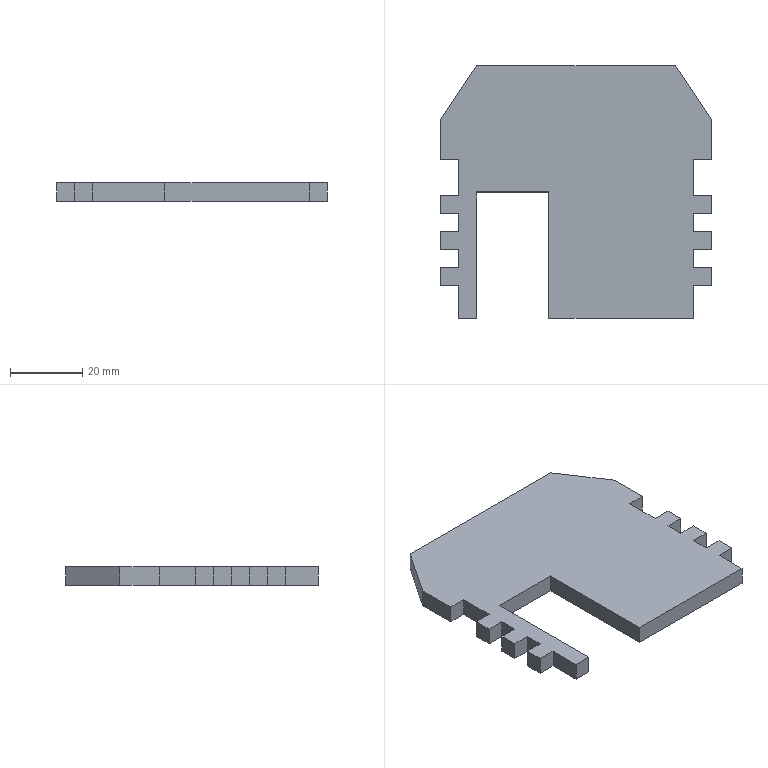Part | SolidWorks | features ICE 5, Attribute 1, Extrusion 1 | 1 solid | 40 faces | box 75 x 70 x 5 mm | volume 20550 mm3 | plane 40
STEP:
#1=CARTESIAN_POINT('',(37.5,-3.5,0.));
#2=VERTEX_POINT('',#1);
#3=CARTESIAN_POINT('',(37.5,1.5,0.));
#4=VERTEX_POINT('',#3);
#5=CARTESIAN_POINT('',(37.5,-37.5,0.));
#6=DIRECTION('',(0.,1.,0.));
#7=VECTOR('',#6,1000.);
#8=LINE('',#5,#7);
#9=EDGE_CURVE('',#2,#4,#8,.T.);
#10=ORIENTED_EDGE('',*,*,#9,.T.);
#11=CARTESIAN_POINT('',(37.5,1.5,5.));
#12=VERTEX_POINT('',#11);
#13=CARTESIAN_POINT('',(37.5,1.5,-0.001));
#14=DIRECTION('',(0.,0.,1.));
#15=VECTOR('',#14,1000.);
#16=LINE('',#13,#15);
#17=EDGE_CURVE('',#4,#12,#16,.T.);
#18=ORIENTED_EDGE('',*,*,#17,.T.);
#19=CARTESIAN_POINT('',(37.5,-3.5,5.));
#20=VERTEX_POINT('',#19);
#21=CARTESIAN_POINT('',(37.5,-37.5,5.));
#22=DIRECTION('',(0.,1.,0.));
#23=VECTOR('',#22,1000.);
#24=LINE('',#21,#23);
#25=EDGE_CURVE('',#20,#12,#24,.T.);
#26=ORIENTED_EDGE('',*,*,#25,.F.);
#27=CARTESIAN_POINT('',(37.5,-3.5,-0.001));
#28=DIRECTION('',(0.,0.,1.));
#29=VECTOR('',#28,1000.);
#30=LINE('',#27,#29);
#31=EDGE_CURVE('',#2,#20,#30,.T.);
#32=ORIENTED_EDGE('',*,*,#31,.F.);
#33=EDGE_LOOP('',(#10,#18,#26,#32));
#34=FACE_OUTER_BOUND('',#33,.T.);
#35=CARTESIAN_POINT('',(37.5,-37.5,5.));
#36=DIRECTION('',(-1.,0.,0.));
#37=DIRECTION('',(0.,0.,1.));
#38=AXIS2_PLACEMENT_3D('',#35,#36,#37);
#39=PLANE('',#38);
#40=ADVANCED_FACE('',(#34),#39,.F.);
#41=CARTESIAN_POINT('',(37.5,-13.5,0.));
#42=VERTEX_POINT('',#41);
#43=CARTESIAN_POINT('',(37.5,-8.5,0.));
#44=VERTEX_POINT('',#43);
#45=CARTESIAN_POINT('',(37.5,-37.5,0.));
#46=DIRECTION('',(0.,1.,0.));
#47=VECTOR('',#46,1000.);
#48=LINE('',#45,#47);
#49=EDGE_CURVE('',#42,#44,#48,.T.);
#50=ORIENTED_EDGE('',*,*,#49,.T.);
#51=CARTESIAN_POINT('',(37.5,-8.5,5.));
#52=VERTEX_POINT('',#51);
#53=CARTESIAN_POINT('',(37.5,-8.5,-0.001));
#54=DIRECTION('',(0.,0.,1.));
#55=VECTOR('',#54,1000.);
#56=LINE('',#53,#55);
#57=EDGE_CURVE('',#44,#52,#56,.T.);
#58=ORIENTED_EDGE('',*,*,#57,.T.);
#59=CARTESIAN_POINT('',(37.5,-13.5,5.));
#60=VERTEX_POINT('',#59);
#61=CARTESIAN_POINT('',(37.5,-37.5,5.));
#62=DIRECTION('',(0.,1.,0.));
#63=VECTOR('',#62,1000.);
#64=LINE('',#61,#63);
#65=EDGE_CURVE('',#60,#52,#64,.T.);
#66=ORIENTED_EDGE('',*,*,#65,.F.);
#67=CARTESIAN_POINT('',(37.5,-13.5,-0.001));
#68=DIRECTION('',(0.,0.,1.));
#69=VECTOR('',#68,1000.);
#70=LINE('',#67,#69);
#71=EDGE_CURVE('',#42,#60,#70,.T.);
#72=ORIENTED_EDGE('',*,*,#71,.F.);
#73=EDGE_LOOP('',(#50,#58,#66,#72));
#74=FACE_OUTER_BOUND('',#73,.T.);
#75=CARTESIAN_POINT('',(37.5,-37.5,5.));
#76=DIRECTION('',(-1.,0.,0.));
#77=DIRECTION('',(0.,0.,1.));
#78=AXIS2_PLACEMENT_3D('',#75,#76,#77);
#79=PLANE('',#78);
#80=ADVANCED_FACE('',(#74),#79,.F.);
#81=CARTESIAN_POINT('',(37.5,-23.5,5.));
#82=VERTEX_POINT('',#81);
#83=CARTESIAN_POINT('',(37.5,-18.5,5.));
#84=VERTEX_POINT('',#83);
#85=CARTESIAN_POINT('',(37.5,-37.5,5.));
#86=DIRECTION('',(0.,1.,0.));
#87=VECTOR('',#86,1000.);
#88=LINE('',#85,#87);
#89=EDGE_CURVE('',#82,#84,#88,.T.);
#90=ORIENTED_EDGE('',*,*,#89,.F.);
#91=CARTESIAN_POINT('',(37.5,-23.5,0.));
#92=VERTEX_POINT('',#91);
#93=CARTESIAN_POINT('',(37.5,-23.5,-0.001));
#94=DIRECTION('',(0.,0.,1.));
#95=VECTOR('',#94,1000.);
#96=LINE('',#93,#95);
#97=EDGE_CURVE('',#92,#82,#96,.T.);
#98=ORIENTED_EDGE('',*,*,#97,.F.);
#99=CARTESIAN_POINT('',(37.5,-18.5,0.));
#100=VERTEX_POINT('',#99);
#101=CARTESIAN_POINT('',(37.5,-37.5,0.));
#102=DIRECTION('',(0.,1.,0.));
#103=VECTOR('',#102,1000.);
#104=LINE('',#101,#103);
#105=EDGE_CURVE('',#92,#100,#104,.T.);
#106=ORIENTED_EDGE('',*,*,#105,.T.);
#107=CARTESIAN_POINT('',(37.5,-18.5,-0.001));
#108=DIRECTION('',(0.,0.,1.));
#109=VECTOR('',#108,1000.);
#110=LINE('',#107,#109);
#111=EDGE_CURVE('',#100,#84,#110,.T.);
#112=ORIENTED_EDGE('',*,*,#111,.T.);
#113=EDGE_LOOP('',(#90,#98,#106,#112));
#114=FACE_OUTER_BOUND('',#113,.T.);
#115=CARTESIAN_POINT('',(37.5,-37.5,5.));
#116=DIRECTION('',(-1.,0.,0.));
#117=DIRECTION('',(0.,0.,1.));
#118=AXIS2_PLACEMENT_3D('',#115,#116,#117);
#119=PLANE('',#118);
#120=ADVANCED_FACE('',(#114),#119,.F.);
#121=CARTESIAN_POINT('',(-37.5,-8.5,0.));
#122=VERTEX_POINT('',#121);
#123=CARTESIAN_POINT('',(-37.5,-13.5,0.));
#124=VERTEX_POINT('',#123);
#125=CARTESIAN_POINT('',(-37.5,-37.5,0.));
#126=DIRECTION('',(0.,-1.,0.));
#127=VECTOR('',#126,1000.);
#128=LINE('',#125,#127);
#129=EDGE_CURVE('',#122,#124,#128,.T.);
#130=ORIENTED_EDGE('',*,*,#129,.T.);
#131=CARTESIAN_POINT('',(-37.5,-13.5,5.));
#132=VERTEX_POINT('',#131);
#133=CARTESIAN_POINT('',(-37.5,-13.5,-0.001));
#134=DIRECTION('',(0.,0.,1.));
#135=VECTOR('',#134,1000.);
#136=LINE('',#133,#135);
#137=EDGE_CURVE('',#124,#132,#136,.T.);
#138=ORIENTED_EDGE('',*,*,#137,.T.);
#139=CARTESIAN_POINT('',(-37.5,-8.5,5.));
#140=VERTEX_POINT('',#139);
#141=CARTESIAN_POINT('',(-37.5,-37.5,5.));
#142=DIRECTION('',(0.,-1.,0.));
#143=VECTOR('',#142,1000.);
#144=LINE('',#141,#143);
#145=EDGE_CURVE('',#140,#132,#144,.T.);
#146=ORIENTED_EDGE('',*,*,#145,.F.);
#147=CARTESIAN_POINT('',(-37.5,-8.5,-0.001));
#148=DIRECTION('',(0.,0.,1.));
#149=VECTOR('',#148,1000.);
#150=LINE('',#147,#149);
#151=EDGE_CURVE('',#122,#140,#150,.T.);
#152=ORIENTED_EDGE('',*,*,#151,.F.);
#153=EDGE_LOOP('',(#130,#138,#146,#152));
#154=FACE_OUTER_BOUND('',#153,.T.);
#155=CARTESIAN_POINT('',(-37.5,-37.5,5.));
#156=DIRECTION('',(1.,0.,0.));
#157=DIRECTION('',(0.,0.,-1.));
#158=AXIS2_PLACEMENT_3D('',#155,#156,#157);
#159=PLANE('',#158);
#160=ADVANCED_FACE('',(#154),#159,.F.);
#161=CARTESIAN_POINT('',(-37.5,1.5,0.));
#162=VERTEX_POINT('',#161);
#163=CARTESIAN_POINT('',(-37.5,-3.5,0.));
#164=VERTEX_POINT('',#163);
#165=CARTESIAN_POINT('',(-37.5,-37.5,0.));
#166=DIRECTION('',(0.,-1.,0.));
#167=VECTOR('',#166,1000.);
#168=LINE('',#165,#167);
#169=EDGE_CURVE('',#162,#164,#168,.T.);
#170=ORIENTED_EDGE('',*,*,#169,.T.);
#171=CARTESIAN_POINT('',(-37.5,-3.5,5.));
#172=VERTEX_POINT('',#171);
#173=CARTESIAN_POINT('',(-37.5,-3.5,-0.001));
#174=DIRECTION('',(0.,0.,1.));
#175=VECTOR('',#174,1000.);
#176=LINE('',#173,#175);
#177=EDGE_CURVE('',#164,#172,#176,.T.);
#178=ORIENTED_EDGE('',*,*,#177,.T.);
#179=CARTESIAN_POINT('',(-37.5,1.5,5.));
#180=VERTEX_POINT('',#179);
#181=CARTESIAN_POINT('',(-37.5,-37.5,5.));
#182=DIRECTION('',(0.,-1.,0.));
#183=VECTOR('',#182,1000.);
#184=LINE('',#181,#183);
#185=EDGE_CURVE('',#180,#172,#184,.T.);
#186=ORIENTED_EDGE('',*,*,#185,.F.);
#187=CARTESIAN_POINT('',(-37.5,1.5,-0.001));
#188=DIRECTION('',(0.,0.,1.));
#189=VECTOR('',#188,1000.);
#190=LINE('',#187,#189);
#191=EDGE_CURVE('',#162,#180,#190,.T.);
#192=ORIENTED_EDGE('',*,*,#191,.F.);
#193=EDGE_LOOP('',(#170,#178,#186,#192));
#194=FACE_OUTER_BOUND('',#193,.T.);
#195=CARTESIAN_POINT('',(-37.5,-37.5,5.));
#196=DIRECTION('',(1.,0.,0.));
#197=DIRECTION('',(0.,0.,-1.));
#198=AXIS2_PLACEMENT_3D('',#195,#196,#197);
#199=PLANE('',#198);
#200=ADVANCED_FACE('',(#194),#199,.F.);
#201=CARTESIAN_POINT('',(-37.5,22.5,0.));
#202=VERTEX_POINT('',#201);
#203=CARTESIAN_POINT('',(-37.5,11.5,0.));
#204=VERTEX_POINT('',#203);
#205=CARTESIAN_POINT('',(-37.5,-37.5,0.));
#206=DIRECTION('',(0.,-1.,0.));
#207=VECTOR('',#206,1000.);
#208=LINE('',#205,#207);
#209=EDGE_CURVE('',#202,#204,#208,.T.);
#210=ORIENTED_EDGE('',*,*,#209,.T.);
#211=CARTESIAN_POINT('',(-37.5,11.5,5.));
#212=VERTEX_POINT('',#211);
#213=CARTESIAN_POINT('',(-37.5,11.5,-0.001));
#214=DIRECTION('',(0.,0.,1.));
#215=VECTOR('',#214,1000.);
#216=LINE('',#213,#215);
#217=EDGE_CURVE('',#204,#212,#216,.T.);
#218=ORIENTED_EDGE('',*,*,#217,.T.);
#219=CARTESIAN_POINT('',(-37.5,22.5,5.));
#220=VERTEX_POINT('',#219);
#221=CARTESIAN_POINT('',(-37.5,-37.5,5.));
#222=DIRECTION('',(0.,-1.,0.));
#223=VECTOR('',#222,1000.);
#224=LINE('',#221,#223);
#225=EDGE_CURVE('',#220,#212,#224,.T.);
#226=ORIENTED_EDGE('',*,*,#225,.F.);
#227=CARTESIAN_POINT('',(-37.5,22.5,0.));
#228=DIRECTION('',(0.,0.,1.));
#229=VECTOR('',#228,1000.);
#230=LINE('',#227,#229);
#231=EDGE_CURVE('',#202,#220,#230,.T.);
#232=ORIENTED_EDGE('',*,*,#231,.F.);
#233=EDGE_LOOP('',(#210,#218,#226,#232));
#234=FACE_OUTER_BOUND('',#233,.T.);
#235=CARTESIAN_POINT('',(-37.5,-37.5,5.));
#236=DIRECTION('',(1.,0.,0.));
#237=DIRECTION('',(0.,0.,-1.));
#238=AXIS2_PLACEMENT_3D('',#235,#236,#237);
#239=PLANE('',#238);
#240=ADVANCED_FACE('',(#234),#239,.F.);
#241=CARTESIAN_POINT('',(-37.5,-18.5,0.));
#242=VERTEX_POINT('',#241);
#243=CARTESIAN_POINT('',(-37.5,-23.5,0.));
#244=VERTEX_POINT('',#243);
#245=CARTESIAN_POINT('',(-37.5,-37.5,0.));
#246=DIRECTION('',(0.,-1.,0.));
#247=VECTOR('',#246,1000.);
#248=LINE('',#245,#247);
#249=EDGE_CURVE('',#242,#244,#248,.T.);
#250=ORIENTED_EDGE('',*,*,#249,.T.);
#251=CARTESIAN_POINT('',(-37.5,-23.5,5.));
#252=VERTEX_POINT('',#251);
#253=CARTESIAN_POINT('',(-37.5,-23.5,-0.001));
#254=DIRECTION('',(0.,0.,1.));
#255=VECTOR('',#254,1000.);
#256=LINE('',#253,#255);
#257=EDGE_CURVE('',#244,#252,#256,.T.);
#258=ORIENTED_EDGE('',*,*,#257,.T.);
#259=CARTESIAN_POINT('',(-37.5,-18.5,5.));
#260=VERTEX_POINT('',#259);
#261=CARTESIAN_POINT('',(-37.5,-37.5,5.));
#262=DIRECTION('',(0.,-1.,0.));
#263=VECTOR('',#262,1000.);
#264=LINE('',#261,#263);
#265=EDGE_CURVE('',#260,#252,#264,.T.);
#266=ORIENTED_EDGE('',*,*,#265,.F.);
#267=CARTESIAN_POINT('',(-37.5,-18.5,-0.001));
#268=DIRECTION('',(0.,0.,1.));
#269=VECTOR('',#268,1000.);
#270=LINE('',#267,#269);
#271=EDGE_CURVE('',#242,#260,#270,.T.);
#272=ORIENTED_EDGE('',*,*,#271,.F.);
#273=EDGE_LOOP('',(#250,#258,#266,#272));
#274=FACE_OUTER_BOUND('',#273,.T.);
#275=CARTESIAN_POINT('',(-37.5,-37.5,5.));
#276=DIRECTION('',(1.,0.,0.));
#277=DIRECTION('',(0.,0.,-1.));
#278=AXIS2_PLACEMENT_3D('',#275,#276,#277);
#279=PLANE('',#278);
#280=ADVANCED_FACE('',(#274),#279,.F.);
#281=CARTESIAN_POINT('',(37.5,11.5,5.));
#282=VERTEX_POINT('',#281);
#283=CARTESIAN_POINT('',(37.5,22.5,5.));
#284=VERTEX_POINT('',#283);
#285=CARTESIAN_POINT('',(37.5,-37.5,5.));
#286=DIRECTION('',(0.,1.,0.));
#287=VECTOR('',#286,1000.);
#288=LINE('',#285,#287);
#289=EDGE_CURVE('',#282,#284,#288,.T.);
#290=ORIENTED_EDGE('',*,*,#289,.F.);
#291=CARTESIAN_POINT('',(37.5,11.5,0.));
#292=VERTEX_POINT('',#291);
#293=CARTESIAN_POINT('',(37.5,11.5,-0.001));
#294=DIRECTION('',(0.,0.,1.));
#295=VECTOR('',#294,1000.);
#296=LINE('',#293,#295);
#297=EDGE_CURVE('',#292,#282,#296,.T.);
#298=ORIENTED_EDGE('',*,*,#297,.F.);
#299=CARTESIAN_POINT('',(37.5,22.5,0.));
#300=VERTEX_POINT('',#299);
#301=CARTESIAN_POINT('',(37.5,-37.5,0.));
#302=DIRECTION('',(0.,1.,0.));
#303=VECTOR('',#302,1000.);
#304=LINE('',#301,#303);
#305=EDGE_CURVE('',#292,#300,#304,.T.);
#306=ORIENTED_EDGE('',*,*,#305,.T.);
#307=CARTESIAN_POINT('',(37.5,22.5,0.));
#308=DIRECTION('',(0.,0.,1.));
#309=VECTOR('',#308,1000.);
#310=LINE('',#307,#309);
#311=EDGE_CURVE('',#300,#284,#310,.T.);
#312=ORIENTED_EDGE('',*,*,#311,.T.);
#313=EDGE_LOOP('',(#290,#298,#306,#312));
#314=FACE_OUTER_BOUND('',#313,.T.);
#315=CARTESIAN_POINT('',(37.5,-37.5,5.));
#316=DIRECTION('',(-1.,0.,0.));
#317=DIRECTION('',(0.,0.,1.));
#318=AXIS2_PLACEMENT_3D('',#315,#316,#317);
#319=PLANE('',#318);
#320=ADVANCED_FACE('',(#314),#319,.F.);
#321=CARTESIAN_POINT('',(27.5,37.5,0.));
#322=VERTEX_POINT('',#321);
#323=CARTESIAN_POINT('',(-27.5,37.5,0.));
#324=VERTEX_POINT('',#323);
#325=CARTESIAN_POINT('',(37.5,37.5,0.));
#326=DIRECTION('',(-1.,0.,0.));
#327=VECTOR('',#326,1000.);
#328=LINE('',#325,#327);
#329=EDGE_CURVE('',#322,#324,#328,.T.);
#330=ORIENTED_EDGE('',*,*,#329,.T.);
#331=CARTESIAN_POINT('',(-27.5,37.5,5.));
#332=VERTEX_POINT('',#331);
#333=CARTESIAN_POINT('',(-27.5,37.5,0.));
#334=DIRECTION('',(0.,0.,1.));
#335=VECTOR('',#334,1000.);
#336=LINE('',#333,#335);
#337=EDGE_CURVE('',#324,#332,#336,.T.);
#338=ORIENTED_EDGE('',*,*,#337,.T.);
#339=CARTESIAN_POINT('',(27.5,37.5,5.));
#340=VERTEX_POINT('',#339);
#341=CARTESIAN_POINT('',(37.5,37.5,5.));
#342=DIRECTION('',(-1.,0.,0.));
#343=VECTOR('',#342,1000.);
#344=LINE('',#341,#343);
#345=EDGE_CURVE('',#340,#332,#344,.T.);
#346=ORIENTED_EDGE('',*,*,#345,.F.);
#347=CARTESIAN_POINT('',(27.5,37.5,0.));
#348=DIRECTION('',(0.,0.,1.));
#349=VECTOR('',#348,1000.);
#350=LINE('',#347,#349);
#351=EDGE_CURVE('',#322,#340,#350,.T.);
#352=ORIENTED_EDGE('',*,*,#351,.F.);
#353=EDGE_LOOP('',(#330,#338,#346,#352));
#354=FACE_OUTER_BOUND('',#353,.T.);
#355=CARTESIAN_POINT('',(37.5,37.5,5.));
#356=DIRECTION('',(0.,-1.,0.));
#357=DIRECTION('',(1.,0.,0.));
#358=AXIS2_PLACEMENT_3D('',#355,#356,#357);
#359=PLANE('',#358);
#360=ADVANCED_FACE('',(#354),#359,.F.);
#361=CARTESIAN_POINT('',(32.5,-32.5,5.));
#362=VERTEX_POINT('',#361);
#363=CARTESIAN_POINT('',(-7.5,-32.5,5.));
#364=VERTEX_POINT('',#363);
#365=CARTESIAN_POINT('',(-32.5,-32.5,5.));
#366=DIRECTION('',(-1.,0.,0.));
#367=VECTOR('',#366,1000.);
#368=LINE('',#365,#367);
#369=EDGE_CURVE('',#362,#364,#368,.T.);
#370=ORIENTED_EDGE('',*,*,#369,.F.);
#371=CARTESIAN_POINT('',(32.5,-23.5,5.));
#372=VERTEX_POINT('',#371);
#373=CARTESIAN_POINT('',(32.5,-37.5,5.));
#374=DIRECTION('',(0.,-1.,0.));
#375=VECTOR('',#374,1000.);
#376=LINE('',#373,#375);
#377=EDGE_CURVE('',#372,#362,#376,.T.);
#378=ORIENTED_EDGE('',*,*,#377,.F.);
#379=CARTESIAN_POINT('',(37.5,-23.5,5.));
#380=DIRECTION('',(-1.,0.,0.));
#381=VECTOR('',#380,1000.);
#382=LINE('',#379,#381);
#383=EDGE_CURVE('',#82,#372,#382,.T.);
#384=ORIENTED_EDGE('',*,*,#383,.F.);
#385=ORIENTED_EDGE('',*,*,#89,.T.);
#386=CARTESIAN_POINT('',(32.5,-18.5,5.));
#387=VERTEX_POINT('',#386);
#388=CARTESIAN_POINT('',(37.5,-18.5,5.));
#389=DIRECTION('',(1.,0.,0.));
#390=VECTOR('',#389,1000.);
#391=LINE('',#388,#390);
#392=EDGE_CURVE('',#387,#84,#391,.T.);
#393=ORIENTED_EDGE('',*,*,#392,.F.);
#394=CARTESIAN_POINT('',(32.5,-13.5,5.));
#395=VERTEX_POINT('',#394);
#396=CARTESIAN_POINT('',(32.5,-18.5,5.));
#397=DIRECTION('',(0.,-1.,0.));
#398=VECTOR('',#397,1000.);
#399=LINE('',#396,#398);
#400=EDGE_CURVE('',#395,#387,#399,.T.);
#401=ORIENTED_EDGE('',*,*,#400,.F.);
#402=CARTESIAN_POINT('',(37.5,-13.5,5.));
#403=DIRECTION('',(-1.,0.,0.));
#404=VECTOR('',#403,1000.);
#405=LINE('',#402,#404);
#406=EDGE_CURVE('',#60,#395,#405,.T.);
#407=ORIENTED_EDGE('',*,*,#406,.F.);
#408=ORIENTED_EDGE('',*,*,#65,.T.);
#409=CARTESIAN_POINT('',(32.5,-8.5,5.));
#410=VERTEX_POINT('',#409);
#411=CARTESIAN_POINT('',(37.5,-8.5,5.));
#412=DIRECTION('',(1.,0.,0.));
#413=VECTOR('',#412,1000.);
#414=LINE('',#411,#413);
#415=EDGE_CURVE('',#410,#52,#414,.T.);
#416=ORIENTED_EDGE('',*,*,#415,.F.);
#417=CARTESIAN_POINT('',(32.5,-3.5,5.));
#418=VERTEX_POINT('',#417);
#419=CARTESIAN_POINT('',(32.5,-8.5,5.));
#420=DIRECTION('',(0.,-1.,0.));
#421=VECTOR('',#420,1000.);
#422=LINE('',#419,#421);
#423=EDGE_CURVE('',#418,#410,#422,.T.);
#424=ORIENTED_EDGE('',*,*,#423,.F.);
#425=CARTESIAN_POINT('',(37.5,-3.5,5.));
#426=DIRECTION('',(-1.,0.,0.));
#427=VECTOR('',#426,1000.);
#428=LINE('',#425,#427);
#429=EDGE_CURVE('',#20,#418,#428,.T.);
#430=ORIENTED_EDGE('',*,*,#429,.F.);
#431=ORIENTED_EDGE('',*,*,#25,.T.);
#432=CARTESIAN_POINT('',(32.5,1.5,5.));
#433=VERTEX_POINT('',#432);
#434=CARTESIAN_POINT('',(37.5,1.5,5.));
#435=DIRECTION('',(1.,0.,0.));
#436=VECTOR('',#435,1000.);
#437=LINE('',#434,#436);
#438=EDGE_CURVE('',#433,#12,#437,.T.);
#439=ORIENTED_EDGE('',*,*,#438,.F.);
#440=CARTESIAN_POINT('',(32.5,11.5,5.));
#441=VERTEX_POINT('',#440);
#442=CARTESIAN_POINT('',(32.5,1.5,5.));
#443=DIRECTION('',(0.,-1.,0.));
#444=VECTOR('',#443,1000.);
#445=LINE('',#442,#444);
#446=EDGE_CURVE('',#441,#433,#445,.T.);
#447=ORIENTED_EDGE('',*,*,#446,.F.);
#448=CARTESIAN_POINT('',(37.5,11.5,5.));
#449=DIRECTION('',(-1.,0.,0.));
#450=VECTOR('',#449,1000.);
#451=LINE('',#448,#450);
#452=EDGE_CURVE('',#282,#441,#451,.T.);
#453=ORIENTED_EDGE('',*,*,#452,.F.);
#454=ORIENTED_EDGE('',*,*,#289,.T.);
#455=CARTESIAN_POINT('',(27.5,37.5,5.));
#456=DIRECTION('',(0.5547,-0.8321,0.));
#457=VECTOR('',#456,1000.);
#458=LINE('',#455,#457);
#459=EDGE_CURVE('',#340,#284,#458,.T.);
#460=ORIENTED_EDGE('',*,*,#459,.F.);
#461=ORIENTED_EDGE('',*,*,#345,.T.);
#462=CARTESIAN_POINT('',(-27.5,37.5,5.));
#463=DIRECTION('',(0.5547,0.8321,0.));
#464=VECTOR('',#463,1000.);
#465=LINE('',#462,#464);
#466=EDGE_CURVE('',#220,#332,#465,.T.);
#467=ORIENTED_EDGE('',*,*,#466,.F.);
#468=ORIENTED_EDGE('',*,*,#225,.T.);
#469=CARTESIAN_POINT('',(-32.5,11.5,5.));
#470=VERTEX_POINT('',#469);
#471=CARTESIAN_POINT('',(-37.5,11.5,5.));
#472=DIRECTION('',(-1.,0.,0.));
#473=VECTOR('',#472,1000.);
#474=LINE('',#471,#473);
#475=EDGE_CURVE('',#470,#212,#474,.T.);
#476=ORIENTED_EDGE('',*,*,#475,.F.);
#477=CARTESIAN_POINT('',(-32.5,1.5,5.));
#478=VERTEX_POINT('',#477);
#479=CARTESIAN_POINT('',(-32.5,1.5,5.));
#480=DIRECTION('',(0.,1.,0.));
#481=VECTOR('',#480,1000.);
#482=LINE('',#479,#481);
#483=EDGE_CURVE('',#478,#470,#482,.T.);
#484=ORIENTED_EDGE('',*,*,#483,.F.);
#485=CARTESIAN_POINT('',(-37.5,1.5,5.));
#486=DIRECTION('',(1.,0.,0.));
#487=VECTOR('',#486,1000.);
#488=LINE('',#485,#487);
#489=EDGE_CURVE('',#180,#478,#488,.T.);
#490=ORIENTED_EDGE('',*,*,#489,.F.);
#491=ORIENTED_EDGE('',*,*,#185,.T.);
#492=CARTESIAN_POINT('',(-32.5,-3.5,5.));
#493=VERTEX_POINT('',#492);
#494=CARTESIAN_POINT('',(-37.5,-3.5,5.));
#495=DIRECTION('',(-1.,0.,0.));
#496=VECTOR('',#495,1000.);
#497=LINE('',#494,#496);
#498=EDGE_CURVE('',#493,#172,#497,.T.);
#499=ORIENTED_EDGE('',*,*,#498,.F.);
#500=CARTESIAN_POINT('',(-32.5,-8.5,5.));
#501=VERTEX_POINT('',#500);
#502=CARTESIAN_POINT('',(-32.5,-8.5,5.));
#503=DIRECTION('',(0.,1.,0.));
#504=VECTOR('',#503,1000.);
#505=LINE('',#502,#504);
#506=EDGE_CURVE('',#501,#493,#505,.T.);
#507=ORIENTED_EDGE('',*,*,#506,.F.);
#508=CARTESIAN_POINT('',(-37.5,-8.5,5.));
#509=DIRECTION('',(1.,0.,0.));
#510=VECTOR('',#509,1000.);
#511=LINE('',#508,#510);
#512=EDGE_CURVE('',#140,#501,#511,.T.);
#513=ORIENTED_EDGE('',*,*,#512,.F.);
#514=ORIENTED_EDGE('',*,*,#145,.T.);
#515=CARTESIAN_POINT('',(-32.5,-13.5,5.));
#516=VERTEX_POINT('',#515);
#517=CARTESIAN_POINT('',(-37.5,-13.5,5.));
#518=DIRECTION('',(-1.,0.,0.));
#519=VECTOR('',#518,1000.);
#520=LINE('',#517,#519);
#521=EDGE_CURVE('',#516,#132,#520,.T.);
#522=ORIENTED_EDGE('',*,*,#521,.F.);
#523=CARTESIAN_POINT('',(-32.5,-18.5,5.));
#524=VERTEX_POINT('',#523);
#525=CARTESIAN_POINT('',(-32.5,-18.5,5.));
#526=DIRECTION('',(0.,1.,0.));
#527=VECTOR('',#526,1000.);
#528=LINE('',#525,#527);
#529=EDGE_CURVE('',#524,#516,#528,.T.);
#530=ORIENTED_EDGE('',*,*,#529,.F.);
#531=CARTESIAN_POINT('',(-37.5,-18.5,5.));
#532=DIRECTION('',(1.,0.,0.));
#533=VECTOR('',#532,1000.);
#534=LINE('',#531,#533);
#535=EDGE_CURVE('',#260,#524,#534,.T.);
#536=ORIENTED_EDGE('',*,*,#535,.F.);
#537=ORIENTED_EDGE('',*,*,#265,.T.);
#538=CARTESIAN_POINT('',(-32.5,-23.5,5.));
#539=VERTEX_POINT('',#538);
#540=CARTESIAN_POINT('',(-37.5,-23.5,5.));
#541=DIRECTION('',(-1.,0.,0.));
#542=VECTOR('',#541,1000.);
#543=LINE('',#540,#542);
#544=EDGE_CURVE('',#539,#252,#543,.T.);
#545=ORIENTED_EDGE('',*,*,#544,.F.);
#546=CARTESIAN_POINT('',(-32.5,-32.5,5.));
#547=VERTEX_POINT('',#546);
#548=CARTESIAN_POINT('',(-32.5,-37.5,5.));
#549=DIRECTION('',(0.,1.,0.));
#550=VECTOR('',#549,1000.);
#551=LINE('',#548,#550);
#552=EDGE_CURVE('',#547,#539,#551,.T.);
#553=ORIENTED_EDGE('',*,*,#552,.F.);
#554=CARTESIAN_POINT('',(-27.5,-32.5,5.));
#555=VERTEX_POINT('',#554);
#556=CARTESIAN_POINT('',(-32.5,-32.5,5.));
#557=DIRECTION('',(-1.,0.,0.));
#558=VECTOR('',#557,1000.);
#559=LINE('',#556,#558);
#560=EDGE_CURVE('',#555,#547,#559,.T.);
#561=ORIENTED_EDGE('',*,*,#560,.F.);
#562=CARTESIAN_POINT('',(-27.5,2.5,5.));
#563=VERTEX_POINT('',#562);
#564=CARTESIAN_POINT('',(-27.5,-37.5,5.));
#565=DIRECTION('',(0.,-1.,0.));
#566=VECTOR('',#565,1000.);
#567=LINE('',#564,#566);
#568=EDGE_CURVE('',#563,#555,#567,.T.);
#569=ORIENTED_EDGE('',*,*,#568,.F.);
#570=CARTESIAN_POINT('',(-7.5,2.5,5.));
#571=VERTEX_POINT('',#570);
#572=CARTESIAN_POINT('',(-27.5,2.5,5.));
#573=DIRECTION('',(-1.,0.,0.));
#574=VECTOR('',#573,1000.);
#575=LINE('',#572,#574);
#576=EDGE_CURVE('',#571,#563,#575,.T.);
#577=ORIENTED_EDGE('',*,*,#576,.F.);
#578=CARTESIAN_POINT('',(-7.5,-37.5,5.));
#579=DIRECTION('',(0.,1.,0.));
#580=VECTOR('',#579,1000.);
#581=LINE('',#578,#580);
#582=EDGE_CURVE('',#364,#571,#581,.T.);
#583=ORIENTED_EDGE('',*,*,#582,.F.);
#584=EDGE_LOOP('',(#370,#378,#384,#385,#393,#401,#407,#408,#416,#424,#430,#431,#439,#447,#453,#454,#460,#461,#467,#468,#476,#484,#490,#491,#499,#507,#513,#514,#522,#530,#536,#537,#545,#553,#561,#569,#577,#583));
#585=FACE_OUTER_BOUND('',#584,.T.);
#586=CARTESIAN_POINT('',(0.,0.,5.));
#587=DIRECTION('',(0.,0.,1.));
#588=DIRECTION('',(1.,0.,0.));
#589=AXIS2_PLACEMENT_3D('',#586,#587,#588);
#590=PLANE('',#589);
#591=ADVANCED_FACE('',(#585),#590,.T.);
#592=CARTESIAN_POINT('',(32.5,-32.5,0.));
#593=VERTEX_POINT('',#592);
#594=CARTESIAN_POINT('',(32.5,-23.5,0.));
#595=VERTEX_POINT('',#594);
#596=CARTESIAN_POINT('',(32.5,-37.5,0.));
#597=DIRECTION('',(0.,1.,0.));
#598=VECTOR('',#597,1000.);
#599=LINE('',#596,#598);
#600=EDGE_CURVE('',#593,#595,#599,.T.);
#601=ORIENTED_EDGE('',*,*,#600,.F.);
#602=CARTESIAN_POINT('',(-7.5,-32.5,0.));
#603=VERTEX_POINT('',#602);
#604=CARTESIAN_POINT('',(0.,-32.5,0.));
#605=DIRECTION('',(-1.,0.,0.));
#606=VECTOR('',#605,1000.);
#607=LINE('',#604,#606);
#608=EDGE_CURVE('',#593,#603,#607,.T.);
#609=ORIENTED_EDGE('',*,*,#608,.T.);
#610=CARTESIAN_POINT('',(-7.5,2.5,0.));
#611=VERTEX_POINT('',#610);
#612=CARTESIAN_POINT('',(-7.5,-37.5,0.));
#613=DIRECTION('',(0.,1.,0.));
#614=VECTOR('',#613,1000.);
#615=LINE('',#612,#614);
#616=EDGE_CURVE('',#603,#611,#615,.T.);
#617=ORIENTED_EDGE('',*,*,#616,.T.);
#618=CARTESIAN_POINT('',(-27.5,2.5,0.));
#619=VERTEX_POINT('',#618);
#620=CARTESIAN_POINT('',(-27.5,2.5,0.));
#621=DIRECTION('',(-1.,0.,0.));
#622=VECTOR('',#621,1000.);
#623=LINE('',#620,#622);
#624=EDGE_CURVE('',#611,#619,#623,.T.);
#625=ORIENTED_EDGE('',*,*,#624,.T.);
#626=CARTESIAN_POINT('',(-27.5,-32.5,0.));
#627=VERTEX_POINT('',#626);
#628=CARTESIAN_POINT('',(-27.5,-37.5,0.));
#629=DIRECTION('',(0.,-1.,0.));
#630=VECTOR('',#629,1000.);
#631=LINE('',#628,#630);
#632=EDGE_CURVE('',#619,#627,#631,.T.);
#633=ORIENTED_EDGE('',*,*,#632,.T.);
#634=CARTESIAN_POINT('',(-32.5,-32.5,0.));
#635=VERTEX_POINT('',#634);
#636=CARTESIAN_POINT('',(0.,-32.5,0.));
#637=DIRECTION('',(-1.,0.,0.));
#638=VECTOR('',#637,1000.);
#639=LINE('',#636,#638);
#640=EDGE_CURVE('',#627,#635,#639,.T.);
#641=ORIENTED_EDGE('',*,*,#640,.T.);
#642=CARTESIAN_POINT('',(-32.5,-23.5,0.));
#643=VERTEX_POINT('',#642);
#644=CARTESIAN_POINT('',(-32.5,-37.5,0.));
#645=DIRECTION('',(0.,-1.,0.));
#646=VECTOR('',#645,1000.);
#647=LINE('',#644,#646);
#648=EDGE_CURVE('',#643,#635,#647,.T.);
#649=ORIENTED_EDGE('',*,*,#648,.F.);
#650=CARTESIAN_POINT('',(-37.5,-23.5,0.));
#651=DIRECTION('',(1.,0.,0.));
#652=VECTOR('',#651,1000.);
#653=LINE('',#650,#652);
#654=EDGE_CURVE('',#244,#643,#653,.T.);
#655=ORIENTED_EDGE('',*,*,#654,.F.);
#656=ORIENTED_EDGE('',*,*,#249,.F.);
#657=CARTESIAN_POINT('',(-32.5,-18.5,0.));
#658=VERTEX_POINT('',#657);
#659=CARTESIAN_POINT('',(-37.5,-18.5,0.));
#660=DIRECTION('',(-1.,0.,0.));
#661=VECTOR('',#660,1000.);
#662=LINE('',#659,#661);
#663=EDGE_CURVE('',#658,#242,#662,.T.);
#664=ORIENTED_EDGE('',*,*,#663,.F.);
#665=CARTESIAN_POINT('',(-32.5,-13.5,0.));
#666=VERTEX_POINT('',#665);
#667=CARTESIAN_POINT('',(-32.5,-18.5,0.));
#668=DIRECTION('',(0.,-1.,0.));
#669=VECTOR('',#668,1000.);
#670=LINE('',#667,#669);
#671=EDGE_CURVE('',#666,#658,#670,.T.);
#672=ORIENTED_EDGE('',*,*,#671,.F.);
#673=CARTESIAN_POINT('',(-37.5,-13.5,0.));
#674=DIRECTION('',(1.,0.,0.));
#675=VECTOR('',#674,1000.);
#676=LINE('',#673,#675);
#677=EDGE_CURVE('',#124,#666,#676,.T.);
#678=ORIENTED_EDGE('',*,*,#677,.F.);
#679=ORIENTED_EDGE('',*,*,#129,.F.);
#680=CARTESIAN_POINT('',(-32.5,-8.5,0.));
#681=VERTEX_POINT('',#680);
#682=CARTESIAN_POINT('',(-37.5,-8.5,0.));
#683=DIRECTION('',(-1.,0.,0.));
#684=VECTOR('',#683,1000.);
#685=LINE('',#682,#684);
#686=EDGE_CURVE('',#681,#122,#685,.T.);
#687=ORIENTED_EDGE('',*,*,#686,.F.);
#688=CARTESIAN_POINT('',(-32.5,-3.5,0.));
#689=VERTEX_POINT('',#688);
#690=CARTESIAN_POINT('',(-32.5,-8.5,0.));
#691=DIRECTION('',(0.,-1.,0.));
#692=VECTOR('',#691,1000.);
#693=LINE('',#690,#692);
#694=EDGE_CURVE('',#689,#681,#693,.T.);
#695=ORIENTED_EDGE('',*,*,#694,.F.);
#696=CARTESIAN_POINT('',(-37.5,-3.5,0.));
#697=DIRECTION('',(1.,0.,0.));
#698=VECTOR('',#697,1000.);
#699=LINE('',#696,#698);
#700=EDGE_CURVE('',#164,#689,#699,.T.);
#701=ORIENTED_EDGE('',*,*,#700,.F.);
#702=ORIENTED_EDGE('',*,*,#169,.F.);
#703=CARTESIAN_POINT('',(-32.5,1.5,0.));
#704=VERTEX_POINT('',#703);
#705=CARTESIAN_POINT('',(-37.5,1.5,0.));
#706=DIRECTION('',(-1.,0.,0.));
#707=VECTOR('',#706,1000.);
#708=LINE('',#705,#707);
#709=EDGE_CURVE('',#704,#162,#708,.T.);
#710=ORIENTED_EDGE('',*,*,#709,.F.);
#711=CARTESIAN_POINT('',(-32.5,11.5,0.));
#712=VERTEX_POINT('',#711);
#713=CARTESIAN_POINT('',(-32.5,1.5,0.));
#714=DIRECTION('',(0.,-1.,0.));
#715=VECTOR('',#714,1000.);
#716=LINE('',#713,#715);
#717=EDGE_CURVE('',#712,#704,#716,.T.);
#718=ORIENTED_EDGE('',*,*,#717,.F.);
#719=CARTESIAN_POINT('',(-37.5,11.5,0.));
#720=DIRECTION('',(1.,0.,0.));
#721=VECTOR('',#720,1000.);
#722=LINE('',#719,#721);
#723=EDGE_CURVE('',#204,#712,#722,.T.);
#724=ORIENTED_EDGE('',*,*,#723,.F.);
#725=ORIENTED_EDGE('',*,*,#209,.F.);
#726=CARTESIAN_POINT('',(-27.5,37.5,0.));
#727=DIRECTION('',(0.5547,0.8321,0.));
#728=VECTOR('',#727,1000.);
#729=LINE('',#726,#728);
#730=EDGE_CURVE('',#202,#324,#729,.T.);
#731=ORIENTED_EDGE('',*,*,#730,.T.);
#732=ORIENTED_EDGE('',*,*,#329,.F.);
#733=CARTESIAN_POINT('',(27.5,37.5,0.));
#734=DIRECTION('',(0.5547,-0.8321,0.));
#735=VECTOR('',#734,1000.);
#736=LINE('',#733,#735);
#737=EDGE_CURVE('',#322,#300,#736,.T.);
#738=ORIENTED_EDGE('',*,*,#737,.T.);
#739=ORIENTED_EDGE('',*,*,#305,.F.);
#740=CARTESIAN_POINT('',(32.5,11.5,0.));
#741=VERTEX_POINT('',#740);
#742=CARTESIAN_POINT('',(37.5,11.5,0.));
#743=DIRECTION('',(1.,0.,0.));
#744=VECTOR('',#743,1000.);
#745=LINE('',#742,#744);
#746=EDGE_CURVE('',#741,#292,#745,.T.);
#747=ORIENTED_EDGE('',*,*,#746,.F.);
#748=CARTESIAN_POINT('',(32.5,1.5,0.));
#749=VERTEX_POINT('',#748);
#750=CARTESIAN_POINT('',(32.5,1.5,0.));
#751=DIRECTION('',(0.,1.,0.));
#752=VECTOR('',#751,1000.);
#753=LINE('',#750,#752);
#754=EDGE_CURVE('',#749,#741,#753,.T.);
#755=ORIENTED_EDGE('',*,*,#754,.F.);
#756=CARTESIAN_POINT('',(37.5,1.5,0.));
#757=DIRECTION('',(-1.,0.,0.));
#758=VECTOR('',#757,1000.);
#759=LINE('',#756,#758);
#760=EDGE_CURVE('',#4,#749,#759,.T.);
#761=ORIENTED_EDGE('',*,*,#760,.F.);
#762=ORIENTED_EDGE('',*,*,#9,.F.);
#763=CARTESIAN_POINT('',(32.5,-3.5,0.));
#764=VERTEX_POINT('',#763);
#765=CARTESIAN_POINT('',(37.5,-3.5,0.));
#766=DIRECTION('',(1.,0.,0.));
#767=VECTOR('',#766,1000.);
#768=LINE('',#765,#767);
#769=EDGE_CURVE('',#764,#2,#768,.T.);
#770=ORIENTED_EDGE('',*,*,#769,.F.);
#771=CARTESIAN_POINT('',(32.5,-8.5,0.));
#772=VERTEX_POINT('',#771);
#773=CARTESIAN_POINT('',(32.5,-8.5,0.));
#774=DIRECTION('',(0.,1.,0.));
#775=VECTOR('',#774,1000.);
#776=LINE('',#773,#775);
#777=EDGE_CURVE('',#772,#764,#776,.T.);
#778=ORIENTED_EDGE('',*,*,#777,.F.);
#779=CARTESIAN_POINT('',(37.5,-8.5,0.));
#780=DIRECTION('',(-1.,0.,0.));
#781=VECTOR('',#780,1000.);
#782=LINE('',#779,#781);
#783=EDGE_CURVE('',#44,#772,#782,.T.);
#784=ORIENTED_EDGE('',*,*,#783,.F.);
#785=ORIENTED_EDGE('',*,*,#49,.F.);
#786=CARTESIAN_POINT('',(32.5,-13.5,0.));
#787=VERTEX_POINT('',#786);
#788=CARTESIAN_POINT('',(37.5,-13.5,0.));
#789=DIRECTION('',(1.,0.,0.));
#790=VECTOR('',#789,1000.);
#791=LINE('',#788,#790);
#792=EDGE_CURVE('',#787,#42,#791,.T.);
#793=ORIENTED_EDGE('',*,*,#792,.F.);
#794=CARTESIAN_POINT('',(32.5,-18.5,0.));
#795=VERTEX_POINT('',#794);
#796=CARTESIAN_POINT('',(32.5,-18.5,0.));
#797=DIRECTION('',(0.,1.,0.));
#798=VECTOR('',#797,1000.);
#799=LINE('',#796,#798);
#800=EDGE_CURVE('',#795,#787,#799,.T.);
#801=ORIENTED_EDGE('',*,*,#800,.F.);
#802=CARTESIAN_POINT('',(37.5,-18.5,0.));
#803=DIRECTION('',(-1.,0.,0.));
#804=VECTOR('',#803,1000.);
#805=LINE('',#802,#804);
#806=EDGE_CURVE('',#100,#795,#805,.T.);
#807=ORIENTED_EDGE('',*,*,#806,.F.);
#808=ORIENTED_EDGE('',*,*,#105,.F.);
#809=CARTESIAN_POINT('',(37.5,-23.5,0.));
#810=DIRECTION('',(1.,0.,0.));
#811=VECTOR('',#810,1000.);
#812=LINE('',#809,#811);
#813=EDGE_CURVE('',#595,#92,#812,.T.);
#814=ORIENTED_EDGE('',*,*,#813,.F.);
#815=EDGE_LOOP('',(#601,#609,#617,#625,#633,#641,#649,#655,#656,#664,#672,#678,#679,#687,#695,#701,#702,#710,#718,#724,#725,#731,#732,#738,#739,#747,#755,#761,#762,#770,#778,#784,#785,#793,#801,#807,#808,#814));
#816=FACE_OUTER_BOUND('',#815,.T.);
#817=CARTESIAN_POINT('',(0.,0.,0.));
#818=DIRECTION('',(0.,0.,1.));
#819=DIRECTION('',(1.,0.,0.));
#820=AXIS2_PLACEMENT_3D('',#817,#818,#819);
#821=PLANE('',#820);
#822=ADVANCED_FACE('',(#816),#821,.F.);
#823=ORIENTED_EDGE('',*,*,#459,.T.);
#824=ORIENTED_EDGE('',*,*,#311,.F.);
#825=ORIENTED_EDGE('',*,*,#737,.F.);
#826=ORIENTED_EDGE('',*,*,#351,.T.);
#827=EDGE_LOOP('',(#823,#824,#825,#826));
#828=FACE_OUTER_BOUND('',#827,.T.);
#829=CARTESIAN_POINT('',(27.5,37.5,0.));
#830=DIRECTION('',(-0.8321,-0.5547,0.));
#831=DIRECTION('',(0.5547,-0.8321,0.));
#832=AXIS2_PLACEMENT_3D('',#829,#830,#831);
#833=PLANE('',#832);
#834=ADVANCED_FACE('',(#828),#833,.F.);
#835=ORIENTED_EDGE('',*,*,#466,.T.);
#836=ORIENTED_EDGE('',*,*,#337,.F.);
#837=ORIENTED_EDGE('',*,*,#730,.F.);
#838=ORIENTED_EDGE('',*,*,#231,.T.);
#839=EDGE_LOOP('',(#835,#836,#837,#838));
#840=FACE_OUTER_BOUND('',#839,.T.);
#841=CARTESIAN_POINT('',(-27.5,37.5,0.));
#842=DIRECTION('',(0.8321,-0.5547,0.));
#843=DIRECTION('',(0.5547,0.8321,0.));
#844=AXIS2_PLACEMENT_3D('',#841,#842,#843);
#845=PLANE('',#844);
#846=ADVANCED_FACE('',(#840),#845,.F.);
#847=ORIENTED_EDGE('',*,*,#568,.T.);
#848=CARTESIAN_POINT('',(-27.5,-32.5,0.));
#849=DIRECTION('',(0.,0.,-1.));
#850=VECTOR('',#849,1000.);
#851=LINE('',#848,#850);
#852=EDGE_CURVE('',#555,#627,#851,.T.);
#853=ORIENTED_EDGE('',*,*,#852,.T.);
#854=ORIENTED_EDGE('',*,*,#632,.F.);
#855=CARTESIAN_POINT('',(-27.5,2.5,0.));
#856=DIRECTION('',(0.,0.,1.));
#857=VECTOR('',#856,1000.);
#858=LINE('',#855,#857);
#859=EDGE_CURVE('',#619,#563,#858,.T.);
#860=ORIENTED_EDGE('',*,*,#859,.T.);
#861=EDGE_LOOP('',(#847,#853,#854,#860));
#862=FACE_OUTER_BOUND('',#861,.T.);
#863=CARTESIAN_POINT('',(-27.5,-37.5,0.));
#864=DIRECTION('',(-1.,0.,0.));
#865=DIRECTION('',(0.,0.,1.));
#866=AXIS2_PLACEMENT_3D('',#863,#864,#865);
#867=PLANE('',#866);
#868=ADVANCED_FACE('',(#862),#867,.F.);
#869=ORIENTED_EDGE('',*,*,#576,.T.);
#870=ORIENTED_EDGE('',*,*,#859,.F.);
#871=ORIENTED_EDGE('',*,*,#624,.F.);
#872=CARTESIAN_POINT('',(-7.5,2.5,0.));
#873=DIRECTION('',(0.,0.,1.));
#874=VECTOR('',#873,1000.);
#875=LINE('',#872,#874);
#876=EDGE_CURVE('',#611,#571,#875,.T.);
#877=ORIENTED_EDGE('',*,*,#876,.T.);
#878=EDGE_LOOP('',(#869,#870,#871,#877));
#879=FACE_OUTER_BOUND('',#878,.T.);
#880=CARTESIAN_POINT('',(-27.5,2.5,0.));
#881=DIRECTION('',(0.,1.,0.));
#882=DIRECTION('',(0.,0.,1.));
#883=AXIS2_PLACEMENT_3D('',#880,#881,#882);
#884=PLANE('',#883);
#885=ADVANCED_FACE('',(#879),#884,.F.);
#886=ORIENTED_EDGE('',*,*,#616,.F.);
#887=CARTESIAN_POINT('',(-7.5,-32.5,0.));
#888=DIRECTION('',(0.,0.,1.));
#889=VECTOR('',#888,1000.);
#890=LINE('',#887,#889);
#891=EDGE_CURVE('',#603,#364,#890,.T.);
#892=ORIENTED_EDGE('',*,*,#891,.T.);
#893=ORIENTED_EDGE('',*,*,#582,.T.);
#894=ORIENTED_EDGE('',*,*,#876,.F.);
#895=EDGE_LOOP('',(#886,#892,#893,#894));
#896=FACE_OUTER_BOUND('',#895,.T.);
#897=CARTESIAN_POINT('',(-7.5,-37.5,0.));
#898=DIRECTION('',(1.,0.,0.));
#899=DIRECTION('',(0.,0.,-1.));
#900=AXIS2_PLACEMENT_3D('',#897,#898,#899);
#901=PLANE('',#900);
#902=ADVANCED_FACE('',(#896),#901,.F.);
#903=ORIENTED_EDGE('',*,*,#723,.T.);
#904=CARTESIAN_POINT('',(-32.5,11.5,-0.001));
#905=DIRECTION('',(0.,0.,1.));
#906=VECTOR('',#905,1000.);
#907=LINE('',#904,#906);
#908=EDGE_CURVE('',#712,#470,#907,.T.);
#909=ORIENTED_EDGE('',*,*,#908,.T.);
#910=ORIENTED_EDGE('',*,*,#475,.T.);
#911=ORIENTED_EDGE('',*,*,#217,.F.);
#912=EDGE_LOOP('',(#903,#909,#910,#911));
#913=FACE_OUTER_BOUND('',#912,.T.);
#914=CARTESIAN_POINT('',(-37.5,11.5,-0.001));
#915=DIRECTION('',(0.,1.,0.));
#916=DIRECTION('',(0.,0.,1.));
#917=AXIS2_PLACEMENT_3D('',#914,#915,#916);
#918=PLANE('',#917);
#919=ADVANCED_FACE('',(#913),#918,.F.);
#920=ORIENTED_EDGE('',*,*,#717,.T.);
#921=CARTESIAN_POINT('',(-32.5,1.5,-0.001));
#922=DIRECTION('',(0.,0.,1.));
#923=VECTOR('',#922,1000.);
#924=LINE('',#921,#923);
#925=EDGE_CURVE('',#704,#478,#924,.T.);
#926=ORIENTED_EDGE('',*,*,#925,.T.);
#927=ORIENTED_EDGE('',*,*,#483,.T.);
#928=ORIENTED_EDGE('',*,*,#908,.F.);
#929=EDGE_LOOP('',(#920,#926,#927,#928));
#930=FACE_OUTER_BOUND('',#929,.T.);
#931=CARTESIAN_POINT('',(-32.5,1.5,-0.001));
#932=DIRECTION('',(1.,0.,0.));
#933=DIRECTION('',(0.,0.,-1.));
#934=AXIS2_PLACEMENT_3D('',#931,#932,#933);
#935=PLANE('',#934);
#936=ADVANCED_FACE('',(#930),#935,.F.);
#937=ORIENTED_EDGE('',*,*,#709,.T.);
#938=ORIENTED_EDGE('',*,*,#191,.T.);
#939=ORIENTED_EDGE('',*,*,#489,.T.);
#940=ORIENTED_EDGE('',*,*,#925,.F.);
#941=EDGE_LOOP('',(#937,#938,#939,#940));
#942=FACE_OUTER_BOUND('',#941,.T.);
#943=CARTESIAN_POINT('',(-37.5,1.5,-0.001));
#944=DIRECTION('',(0.,-1.,0.));
#945=DIRECTION('',(0.,0.,-1.));
#946=AXIS2_PLACEMENT_3D('',#943,#944,#945);
#947=PLANE('',#946);
#948=ADVANCED_FACE('',(#942),#947,.F.);
#949=ORIENTED_EDGE('',*,*,#700,.T.);
#950=CARTESIAN_POINT('',(-32.5,-3.5,-0.001));
#951=DIRECTION('',(0.,0.,1.));
#952=VECTOR('',#951,1000.);
#953=LINE('',#950,#952);
#954=EDGE_CURVE('',#689,#493,#953,.T.);
#955=ORIENTED_EDGE('',*,*,#954,.T.);
#956=ORIENTED_EDGE('',*,*,#498,.T.);
#957=ORIENTED_EDGE('',*,*,#177,.F.);
#958=EDGE_LOOP('',(#949,#955,#956,#957));
#959=FACE_OUTER_BOUND('',#958,.T.);
#960=CARTESIAN_POINT('',(-37.5,-3.5,-0.001));
#961=DIRECTION('',(0.,1.,0.));
#962=DIRECTION('',(0.,0.,1.));
#963=AXIS2_PLACEMENT_3D('',#960,#961,#962);
#964=PLANE('',#963);
#965=ADVANCED_FACE('',(#959),#964,.F.);
#966=ORIENTED_EDGE('',*,*,#694,.T.);
#967=CARTESIAN_POINT('',(-32.5,-8.5,-0.001));
#968=DIRECTION('',(0.,0.,1.));
#969=VECTOR('',#968,1000.);
#970=LINE('',#967,#969);
#971=EDGE_CURVE('',#681,#501,#970,.T.);
#972=ORIENTED_EDGE('',*,*,#971,.T.);
#973=ORIENTED_EDGE('',*,*,#506,.T.);
#974=ORIENTED_EDGE('',*,*,#954,.F.);
#975=EDGE_LOOP('',(#966,#972,#973,#974));
#976=FACE_OUTER_BOUND('',#975,.T.);
#977=CARTESIAN_POINT('',(-32.5,-8.5,-0.001));
#978=DIRECTION('',(1.,0.,0.));
#979=DIRECTION('',(0.,0.,-1.));
#980=AXIS2_PLACEMENT_3D('',#977,#978,#979);
#981=PLANE('',#980);
#982=ADVANCED_FACE('',(#976),#981,.F.);
#983=ORIENTED_EDGE('',*,*,#686,.T.);
#984=ORIENTED_EDGE('',*,*,#151,.T.);
#985=ORIENTED_EDGE('',*,*,#512,.T.);
#986=ORIENTED_EDGE('',*,*,#971,.F.);
#987=EDGE_LOOP('',(#983,#984,#985,#986));
#988=FACE_OUTER_BOUND('',#987,.T.);
#989=CARTESIAN_POINT('',(-37.5,-8.5,-0.001));
#990=DIRECTION('',(0.,-1.,0.));
#991=DIRECTION('',(0.,0.,-1.));
#992=AXIS2_PLACEMENT_3D('',#989,#990,#991);
#993=PLANE('',#992);
#994=ADVANCED_FACE('',(#988),#993,.F.);
#995=ORIENTED_EDGE('',*,*,#677,.T.);
#996=CARTESIAN_POINT('',(-32.5,-13.5,-0.001));
#997=DIRECTION('',(0.,0.,1.));
#998=VECTOR('',#997,1000.);
#999=LINE('',#996,#998);
#1000=EDGE_CURVE('',#666,#516,#999,.T.);
#1001=ORIENTED_EDGE('',*,*,#1000,.T.);
#1002=ORIENTED_EDGE('',*,*,#521,.T.);
#1003=ORIENTED_EDGE('',*,*,#137,.F.);
#1004=EDGE_LOOP('',(#995,#1001,#1002,#1003));
#1005=FACE_OUTER_BOUND('',#1004,.T.);
#1006=CARTESIAN_POINT('',(-37.5,-13.5,-0.001));
#1007=DIRECTION('',(0.,1.,0.));
#1008=DIRECTION('',(0.,0.,1.));
#1009=AXIS2_PLACEMENT_3D('',#1006,#1007,#1008);
#1010=PLANE('',#1009);
#1011=ADVANCED_FACE('',(#1005),#1010,.F.);
#1012=ORIENTED_EDGE('',*,*,#671,.T.);
#1013=CARTESIAN_POINT('',(-32.5,-18.5,-0.001));
#1014=DIRECTION('',(0.,0.,1.));
#1015=VECTOR('',#1014,1000.);
#1016=LINE('',#1013,#1015);
#1017=EDGE_CURVE('',#658,#524,#1016,.T.);
#1018=ORIENTED_EDGE('',*,*,#1017,.T.);
#1019=ORIENTED_EDGE('',*,*,#529,.T.);
#1020=ORIENTED_EDGE('',*,*,#1000,.F.);
#1021=EDGE_LOOP('',(#1012,#1018,#1019,#1020));
#1022=FACE_OUTER_BOUND('',#1021,.T.);
#1023=CARTESIAN_POINT('',(-32.5,-18.5,-0.001));
#1024=DIRECTION('',(1.,0.,0.));
#1025=DIRECTION('',(0.,0.,-1.));
#1026=AXIS2_PLACEMENT_3D('',#1023,#1024,#1025);
#1027=PLANE('',#1026);
#1028=ADVANCED_FACE('',(#1022),#1027,.F.);
#1029=ORIENTED_EDGE('',*,*,#663,.T.);
#1030=ORIENTED_EDGE('',*,*,#271,.T.);
#1031=ORIENTED_EDGE('',*,*,#535,.T.);
#1032=ORIENTED_EDGE('',*,*,#1017,.F.);
#1033=EDGE_LOOP('',(#1029,#1030,#1031,#1032));
#1034=FACE_OUTER_BOUND('',#1033,.T.);
#1035=CARTESIAN_POINT('',(-37.5,-18.5,-0.001));
#1036=DIRECTION('',(0.,-1.,0.));
#1037=DIRECTION('',(0.,0.,-1.));
#1038=AXIS2_PLACEMENT_3D('',#1035,#1036,#1037);
#1039=PLANE('',#1038);
#1040=ADVANCED_FACE('',(#1034),#1039,.F.);
#1041=ORIENTED_EDGE('',*,*,#654,.T.);
#1042=CARTESIAN_POINT('',(-32.5,-23.5,-0.001));
#1043=DIRECTION('',(0.,0.,1.));
#1044=VECTOR('',#1043,1000.);
#1045=LINE('',#1042,#1044);
#1046=EDGE_CURVE('',#643,#539,#1045,.T.);
#1047=ORIENTED_EDGE('',*,*,#1046,.T.);
#1048=ORIENTED_EDGE('',*,*,#544,.T.);
#1049=ORIENTED_EDGE('',*,*,#257,.F.);
#1050=EDGE_LOOP('',(#1041,#1047,#1048,#1049));
#1051=FACE_OUTER_BOUND('',#1050,.T.);
#1052=CARTESIAN_POINT('',(-37.5,-23.5,-0.001));
#1053=DIRECTION('',(0.,1.,0.));
#1054=DIRECTION('',(0.,0.,1.));
#1055=AXIS2_PLACEMENT_3D('',#1052,#1053,#1054);
#1056=PLANE('',#1055);
#1057=ADVANCED_FACE('',(#1051),#1056,.F.);
#1058=ORIENTED_EDGE('',*,*,#648,.T.);
#1059=CARTESIAN_POINT('',(-32.5,-32.5,-5.));
#1060=DIRECTION('',(0.,0.,1.));
#1061=VECTOR('',#1060,1000.);
#1062=LINE('',#1059,#1061);
#1063=EDGE_CURVE('',#635,#547,#1062,.T.);
#1064=ORIENTED_EDGE('',*,*,#1063,.T.);
#1065=ORIENTED_EDGE('',*,*,#552,.T.);
#1066=ORIENTED_EDGE('',*,*,#1046,.F.);
#1067=EDGE_LOOP('',(#1058,#1064,#1065,#1066));
#1068=FACE_OUTER_BOUND('',#1067,.T.);
#1069=CARTESIAN_POINT('',(-32.5,-37.5,-0.001));
#1070=DIRECTION('',(1.,0.,0.));
#1071=DIRECTION('',(0.,0.,-1.));
#1072=AXIS2_PLACEMENT_3D('',#1069,#1070,#1071);
#1073=PLANE('',#1072);
#1074=ADVANCED_FACE('',(#1068),#1073,.F.);
#1075=ORIENTED_EDGE('',*,*,#806,.T.);
#1076=CARTESIAN_POINT('',(32.5,-18.5,-0.001));
#1077=DIRECTION('',(0.,0.,1.));
#1078=VECTOR('',#1077,1000.);
#1079=LINE('',#1076,#1078);
#1080=EDGE_CURVE('',#795,#387,#1079,.T.);
#1081=ORIENTED_EDGE('',*,*,#1080,.T.);
#1082=ORIENTED_EDGE('',*,*,#392,.T.);
#1083=ORIENTED_EDGE('',*,*,#111,.F.);
#1084=EDGE_LOOP('',(#1075,#1081,#1082,#1083));
#1085=FACE_OUTER_BOUND('',#1084,.T.);
#1086=CARTESIAN_POINT('',(37.5,-18.5,-0.001));
#1087=DIRECTION('',(0.,-1.,0.));
#1088=DIRECTION('',(0.,0.,-1.));
#1089=AXIS2_PLACEMENT_3D('',#1086,#1087,#1088);
#1090=PLANE('',#1089);
#1091=ADVANCED_FACE('',(#1085),#1090,.F.);
#1092=ORIENTED_EDGE('',*,*,#800,.T.);
#1093=CARTESIAN_POINT('',(32.5,-13.5,-0.001));
#1094=DIRECTION('',(0.,0.,1.));
#1095=VECTOR('',#1094,1000.);
#1096=LINE('',#1093,#1095);
#1097=EDGE_CURVE('',#787,#395,#1096,.T.);
#1098=ORIENTED_EDGE('',*,*,#1097,.T.);
#1099=ORIENTED_EDGE('',*,*,#400,.T.);
#1100=ORIENTED_EDGE('',*,*,#1080,.F.);
#1101=EDGE_LOOP('',(#1092,#1098,#1099,#1100));
#1102=FACE_OUTER_BOUND('',#1101,.T.);
#1103=CARTESIAN_POINT('',(32.5,-18.5,-0.001));
#1104=DIRECTION('',(-1.,0.,0.));
#1105=DIRECTION('',(0.,-1.,0.));
#1106=AXIS2_PLACEMENT_3D('',#1103,#1104,#1105);
#1107=PLANE('',#1106);
#1108=ADVANCED_FACE('',(#1102),#1107,.F.);
#1109=ORIENTED_EDGE('',*,*,#792,.T.);
#1110=ORIENTED_EDGE('',*,*,#71,.T.);
#1111=ORIENTED_EDGE('',*,*,#406,.T.);
#1112=ORIENTED_EDGE('',*,*,#1097,.F.);
#1113=EDGE_LOOP('',(#1109,#1110,#1111,#1112));
#1114=FACE_OUTER_BOUND('',#1113,.T.);
#1115=CARTESIAN_POINT('',(37.5,-13.5,-0.001));
#1116=DIRECTION('',(0.,1.,0.));
#1117=DIRECTION('',(0.,0.,1.));
#1118=AXIS2_PLACEMENT_3D('',#1115,#1116,#1117);
#1119=PLANE('',#1118);
#1120=ADVANCED_FACE('',(#1114),#1119,.F.);
#1121=ORIENTED_EDGE('',*,*,#783,.T.);
#1122=CARTESIAN_POINT('',(32.5,-8.5,-0.001));
#1123=DIRECTION('',(0.,0.,1.));
#1124=VECTOR('',#1123,1000.);
#1125=LINE('',#1122,#1124);
#1126=EDGE_CURVE('',#772,#410,#1125,.T.);
#1127=ORIENTED_EDGE('',*,*,#1126,.T.);
#1128=ORIENTED_EDGE('',*,*,#415,.T.);
#1129=ORIENTED_EDGE('',*,*,#57,.F.);
#1130=EDGE_LOOP('',(#1121,#1127,#1128,#1129));
#1131=FACE_OUTER_BOUND('',#1130,.T.);
#1132=CARTESIAN_POINT('',(37.5,-8.5,-0.001));
#1133=DIRECTION('',(0.,-1.,0.));
#1134=DIRECTION('',(0.,0.,-1.));
#1135=AXIS2_PLACEMENT_3D('',#1132,#1133,#1134);
#1136=PLANE('',#1135);
#1137=ADVANCED_FACE('',(#1131),#1136,.F.);
#1138=ORIENTED_EDGE('',*,*,#777,.T.);
#1139=CARTESIAN_POINT('',(32.5,-3.5,-0.001));
#1140=DIRECTION('',(0.,0.,1.));
#1141=VECTOR('',#1140,1000.);
#1142=LINE('',#1139,#1141);
#1143=EDGE_CURVE('',#764,#418,#1142,.T.);
#1144=ORIENTED_EDGE('',*,*,#1143,.T.);
#1145=ORIENTED_EDGE('',*,*,#423,.T.);
#1146=ORIENTED_EDGE('',*,*,#1126,.F.);
#1147=EDGE_LOOP('',(#1138,#1144,#1145,#1146));
#1148=FACE_OUTER_BOUND('',#1147,.T.);
#1149=CARTESIAN_POINT('',(32.5,-8.5,-0.001));
#1150=DIRECTION('',(-1.,0.,0.));
#1151=DIRECTION('',(0.,-1.,0.));
#1152=AXIS2_PLACEMENT_3D('',#1149,#1150,#1151);
#1153=PLANE('',#1152);
#1154=ADVANCED_FACE('',(#1148),#1153,.F.);
#1155=ORIENTED_EDGE('',*,*,#769,.T.);
#1156=ORIENTED_EDGE('',*,*,#31,.T.);
#1157=ORIENTED_EDGE('',*,*,#429,.T.);
#1158=ORIENTED_EDGE('',*,*,#1143,.F.);
#1159=EDGE_LOOP('',(#1155,#1156,#1157,#1158));
#1160=FACE_OUTER_BOUND('',#1159,.T.);
#1161=CARTESIAN_POINT('',(37.5,-3.5,-0.001));
#1162=DIRECTION('',(0.,1.,0.));
#1163=DIRECTION('',(0.,0.,1.));
#1164=AXIS2_PLACEMENT_3D('',#1161,#1162,#1163);
#1165=PLANE('',#1164);
#1166=ADVANCED_FACE('',(#1160),#1165,.F.);
#1167=ORIENTED_EDGE('',*,*,#760,.T.);
#1168=CARTESIAN_POINT('',(32.5,1.5,-0.001));
#1169=DIRECTION('',(0.,0.,1.));
#1170=VECTOR('',#1169,1000.);
#1171=LINE('',#1168,#1170);
#1172=EDGE_CURVE('',#749,#433,#1171,.T.);
#1173=ORIENTED_EDGE('',*,*,#1172,.T.);
#1174=ORIENTED_EDGE('',*,*,#438,.T.);
#1175=ORIENTED_EDGE('',*,*,#17,.F.);
#1176=EDGE_LOOP('',(#1167,#1173,#1174,#1175));
#1177=FACE_OUTER_BOUND('',#1176,.T.);
#1178=CARTESIAN_POINT('',(37.5,1.5,-0.001));
#1179=DIRECTION('',(0.,-1.,0.));
#1180=DIRECTION('',(1.,0.,0.));
#1181=AXIS2_PLACEMENT_3D('',#1178,#1179,#1180);
#1182=PLANE('',#1181);
#1183=ADVANCED_FACE('',(#1177),#1182,.F.);
#1184=ORIENTED_EDGE('',*,*,#754,.T.);
#1185=CARTESIAN_POINT('',(32.5,11.5,-0.001));
#1186=DIRECTION('',(0.,0.,1.));
#1187=VECTOR('',#1186,1000.);
#1188=LINE('',#1185,#1187);
#1189=EDGE_CURVE('',#741,#441,#1188,.T.);
#1190=ORIENTED_EDGE('',*,*,#1189,.T.);
#1191=ORIENTED_EDGE('',*,*,#446,.T.);
#1192=ORIENTED_EDGE('',*,*,#1172,.F.);
#1193=EDGE_LOOP('',(#1184,#1190,#1191,#1192));
#1194=FACE_OUTER_BOUND('',#1193,.T.);
#1195=CARTESIAN_POINT('',(32.5,1.5,-0.001));
#1196=DIRECTION('',(-1.,0.,0.));
#1197=DIRECTION('',(0.,0.,1.));
#1198=AXIS2_PLACEMENT_3D('',#1195,#1196,#1197);
#1199=PLANE('',#1198);
#1200=ADVANCED_FACE('',(#1194),#1199,.F.);
#1201=ORIENTED_EDGE('',*,*,#746,.T.);
#1202=ORIENTED_EDGE('',*,*,#297,.T.);
#1203=ORIENTED_EDGE('',*,*,#452,.T.);
#1204=ORIENTED_EDGE('',*,*,#1189,.F.);
#1205=EDGE_LOOP('',(#1201,#1202,#1203,#1204));
#1206=FACE_OUTER_BOUND('',#1205,.T.);
#1207=CARTESIAN_POINT('',(37.5,11.5,-0.001));
#1208=DIRECTION('',(0.,1.,0.));
#1209=DIRECTION('',(0.,0.,1.));
#1210=AXIS2_PLACEMENT_3D('',#1207,#1208,#1209);
#1211=PLANE('',#1210);
#1212=ADVANCED_FACE('',(#1206),#1211,.F.);
#1213=ORIENTED_EDGE('',*,*,#377,.T.);
#1214=CARTESIAN_POINT('',(32.5,-32.5,-0.001));
#1215=DIRECTION('',(0.,0.,-1.));
#1216=VECTOR('',#1215,1000.);
#1217=LINE('',#1214,#1216);
#1218=EDGE_CURVE('',#362,#593,#1217,.T.);
#1219=ORIENTED_EDGE('',*,*,#1218,.T.);
#1220=ORIENTED_EDGE('',*,*,#600,.T.);
#1221=CARTESIAN_POINT('',(32.5,-23.5,-0.001));
#1222=DIRECTION('',(0.,0.,1.));
#1223=VECTOR('',#1222,1000.);
#1224=LINE('',#1221,#1223);
#1225=EDGE_CURVE('',#595,#372,#1224,.T.);
#1226=ORIENTED_EDGE('',*,*,#1225,.T.);
#1227=EDGE_LOOP('',(#1213,#1219,#1220,#1226));
#1228=FACE_OUTER_BOUND('',#1227,.T.);
#1229=CARTESIAN_POINT('',(32.5,-37.5,-0.001));
#1230=DIRECTION('',(-1.,0.,0.));
#1231=DIRECTION('',(0.,0.,1.));
#1232=AXIS2_PLACEMENT_3D('',#1229,#1230,#1231);
#1233=PLANE('',#1232);
#1234=ADVANCED_FACE('',(#1228),#1233,.F.);
#1235=ORIENTED_EDGE('',*,*,#813,.T.);
#1236=ORIENTED_EDGE('',*,*,#97,.T.);
#1237=ORIENTED_EDGE('',*,*,#383,.T.);
#1238=ORIENTED_EDGE('',*,*,#1225,.F.);
#1239=EDGE_LOOP('',(#1235,#1236,#1237,#1238));
#1240=FACE_OUTER_BOUND('',#1239,.T.);
#1241=CARTESIAN_POINT('',(37.5,-23.5,-0.001));
#1242=DIRECTION('',(0.,1.,0.));
#1243=DIRECTION('',(0.,0.,1.));
#1244=AXIS2_PLACEMENT_3D('',#1241,#1242,#1243);
#1245=PLANE('',#1244);
#1246=ADVANCED_FACE('',(#1240),#1245,.F.);
#1247=ORIENTED_EDGE('',*,*,#1218,.F.);
#1248=ORIENTED_EDGE('',*,*,#369,.T.);
#1249=ORIENTED_EDGE('',*,*,#891,.F.);
#1250=ORIENTED_EDGE('',*,*,#608,.F.);
#1251=EDGE_LOOP('',(#1247,#1248,#1249,#1250));
#1252=FACE_OUTER_BOUND('',#1251,.T.);
#1253=CARTESIAN_POINT('',(-32.5,-32.5,-5.));
#1254=DIRECTION('',(0.,1.,0.));
#1255=DIRECTION('',(0.,0.,1.));
#1256=AXIS2_PLACEMENT_3D('',#1253,#1254,#1255);
#1257=PLANE('',#1256);
#1258=ADVANCED_FACE('',(#1252),#1257,.F.);
#1259=ORIENTED_EDGE('',*,*,#852,.F.);
#1260=ORIENTED_EDGE('',*,*,#560,.T.);
#1261=ORIENTED_EDGE('',*,*,#1063,.F.);
#1262=ORIENTED_EDGE('',*,*,#640,.F.);
#1263=EDGE_LOOP('',(#1259,#1260,#1261,#1262));
#1264=FACE_OUTER_BOUND('',#1263,.T.);
#1265=CARTESIAN_POINT('',(-32.5,-32.5,-5.));
#1266=DIRECTION('',(0.,1.,0.));
#1267=DIRECTION('',(0.,0.,1.));
#1268=AXIS2_PLACEMENT_3D('',#1265,#1266,#1267);
#1269=PLANE('',#1268);
#1270=ADVANCED_FACE('',(#1264),#1269,.F.);
#1271=CLOSED_SHELL('',(#40,#80,#120,#160,#200,#240,#280,#320,#360,#591,#822,#834,#846,#868,#885,#902,#919,#936,#948,#965,#982,#994,#1011,#1028,#1040,#1057,#1074,#1091,#1108,#1120,#1137,#1154,#1166,#1183,#1200,#1212,#1234,#1246,#1258,#1270));
#1272=MANIFOLD_SOLID_BREP('',#1271);
#1273=CARTESIAN_POINT('',(0.,0.,0.));
#1274=DIRECTION('',(0.,0.,1.));
#1275=DIRECTION('',(1.,0.,0.));
#1276=AXIS2_PLACEMENT_3D('',#1273,#1274,#1275);
#1277=(LENGTH_UNIT()NAMED_UNIT(*)SI_UNIT(.MILLI.,.METRE.));
#1278=UNCERTAINTY_MEASURE_WITH_UNIT(LENGTH_MEASURE(0.00001),#1277,'','');
#1279=(NAMED_UNIT(*)PLANE_ANGLE_UNIT()SI_UNIT($,.RADIAN.));
#1280=(NAMED_UNIT(*)SI_UNIT($,.STERADIAN.)SOLID_ANGLE_UNIT());
#1281=(GEOMETRIC_REPRESENTATION_CONTEXT(3)GLOBAL_UNCERTAINTY_ASSIGNED_CONTEXT((#1278))GLOBAL_UNIT_ASSIGNED_CONTEXT((#1277,#1279,#1280))REPRESENTATION_CONTEXT('',''));
#1282=ADVANCED_BREP_SHAPE_REPRESENTATION('',(#1272,#1276),#1281);